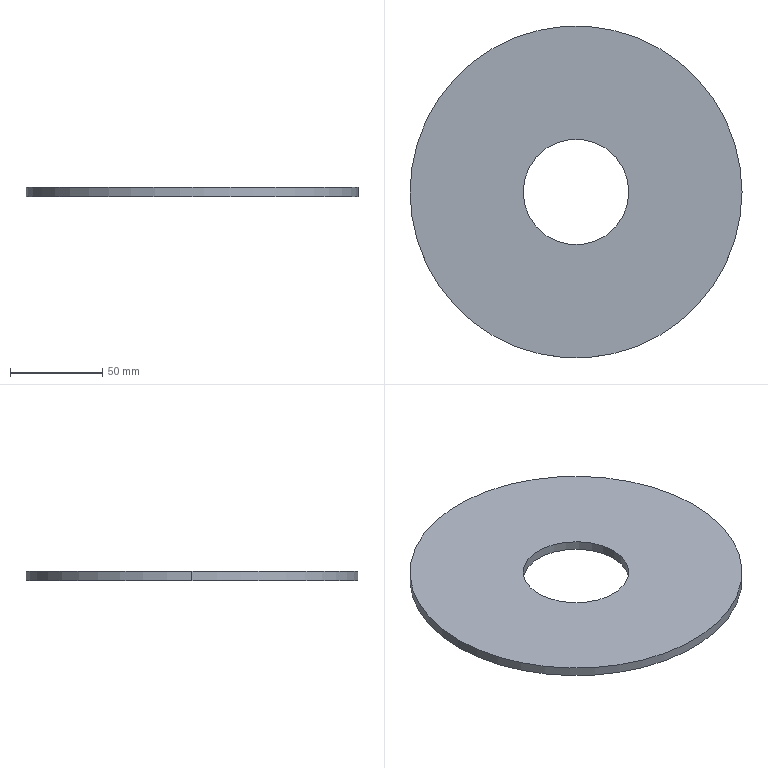Part | SolidWorks | features FlatPattern 1, SMBaseFlange 1, SheetMetal 1 | 1 solid | 6 faces | box 180 x 180 x 5 mm | volume 114341 mm3 | cylinder 4 | plane 2 | commonest cylinder face diameters 57.3 x2 180 x2
STEP:
#1=CARTESIAN_POINT('',(-38.194,24.146,5.));
#2=VERTEX_POINT('',#1);
#3=CARTESIAN_POINT('',(19.106,24.146,5.));
#4=VERTEX_POINT('',#3);
#5=CARTESIAN_POINT('',(-9.544,24.146,5.));
#6=DIRECTION('',(0.,0.,1.));
#7=DIRECTION('',(1.,0.,0.));
#8=AXIS2_PLACEMENT_3D('',#5,#6,#7);
#9=CIRCLE('',#8,28.65);
#10=EDGE_CURVE('',#2,#4,#9,.T.);
#11=ORIENTED_EDGE('',*,*,#10,.T.);
#12=CARTESIAN_POINT('',(19.106,24.146,0.));
#13=VERTEX_POINT('',#12);
#14=CARTESIAN_POINT('',(19.106,24.146,5.));
#15=DIRECTION('',(0.,0.,-1.));
#16=VECTOR('',#15,1000.);
#17=LINE('',#14,#16);
#18=EDGE_CURVE('',#4,#13,#17,.T.);
#19=ORIENTED_EDGE('',*,*,#18,.T.);
#20=CARTESIAN_POINT('',(-38.194,24.146,0.));
#21=VERTEX_POINT('',#20);
#22=CARTESIAN_POINT('',(-9.544,24.146,0.));
#23=DIRECTION('',(0.,0.,1.));
#24=DIRECTION('',(1.,0.,0.));
#25=AXIS2_PLACEMENT_3D('',#22,#23,#24);
#26=CIRCLE('',#25,28.65);
#27=EDGE_CURVE('',#21,#13,#26,.T.);
#28=ORIENTED_EDGE('',*,*,#27,.F.);
#29=CARTESIAN_POINT('',(-38.194,24.146,5.));
#30=DIRECTION('',(0.,0.,-1.));
#31=VECTOR('',#30,1000.);
#32=LINE('',#29,#31);
#33=EDGE_CURVE('',#2,#21,#32,.T.);
#34=ORIENTED_EDGE('',*,*,#33,.F.);
#35=EDGE_LOOP('',(#11,#19,#28,#34));
#36=FACE_OUTER_BOUND('',#35,.T.);
#37=CARTESIAN_POINT('',(-9.544,24.146,5.));
#38=DIRECTION('',(0.,0.,-1.));
#39=DIRECTION('',(-1.,0.,0.));
#40=AXIS2_PLACEMENT_3D('',#37,#38,#39);
#41=CYLINDRICAL_SURFACE('',#40,28.65);
#42=ADVANCED_FACE('',(#36),#41,.F.);
#43=CARTESIAN_POINT('',(80.456,24.146,5.));
#44=VERTEX_POINT('',#43);
#45=CARTESIAN_POINT('',(-99.544,24.146,5.));
#46=VERTEX_POINT('',#45);
#47=CARTESIAN_POINT('',(-9.544,24.146,5.));
#48=DIRECTION('',(0.,0.,1.));
#49=DIRECTION('',(1.,0.,0.));
#50=AXIS2_PLACEMENT_3D('',#47,#48,#49);
#51=CIRCLE('',#50,90.);
#52=EDGE_CURVE('',#44,#46,#51,.T.);
#53=ORIENTED_EDGE('',*,*,#52,.F.);
#54=CARTESIAN_POINT('',(80.456,24.146,0.));
#55=VERTEX_POINT('',#54);
#56=CARTESIAN_POINT('',(80.456,24.146,5.));
#57=DIRECTION('',(0.,0.,-1.));
#58=VECTOR('',#57,1000.);
#59=LINE('',#56,#58);
#60=EDGE_CURVE('',#44,#55,#59,.T.);
#61=ORIENTED_EDGE('',*,*,#60,.T.);
#62=CARTESIAN_POINT('',(-99.544,24.146,0.));
#63=VERTEX_POINT('',#62);
#64=CARTESIAN_POINT('',(-9.544,24.146,0.));
#65=DIRECTION('',(0.,0.,1.));
#66=DIRECTION('',(1.,0.,0.));
#67=AXIS2_PLACEMENT_3D('',#64,#65,#66);
#68=CIRCLE('',#67,90.);
#69=EDGE_CURVE('',#55,#63,#68,.T.);
#70=ORIENTED_EDGE('',*,*,#69,.T.);
#71=CARTESIAN_POINT('',(-99.544,24.146,5.));
#72=DIRECTION('',(0.,0.,-1.));
#73=VECTOR('',#72,1000.);
#74=LINE('',#71,#73);
#75=EDGE_CURVE('',#46,#63,#74,.T.);
#76=ORIENTED_EDGE('',*,*,#75,.F.);
#77=EDGE_LOOP('',(#53,#61,#70,#76));
#78=FACE_OUTER_BOUND('',#77,.T.);
#79=CARTESIAN_POINT('',(-9.544,24.146,5.));
#80=DIRECTION('',(0.,0.,-1.));
#81=DIRECTION('',(-1.,0.,0.));
#82=AXIS2_PLACEMENT_3D('',#79,#80,#81);
#83=CYLINDRICAL_SURFACE('',#82,90.);
#84=ADVANCED_FACE('',(#78),#83,.T.);
#85=CARTESIAN_POINT('',(-9.544,24.146,5.));
#86=DIRECTION('',(0.,0.,1.));
#87=DIRECTION('',(1.,0.,0.));
#88=AXIS2_PLACEMENT_3D('',#85,#86,#87);
#89=CIRCLE('',#88,90.);
#90=EDGE_CURVE('',#46,#44,#89,.T.);
#91=ORIENTED_EDGE('',*,*,#90,.T.);
#92=ORIENTED_EDGE('',*,*,#52,.T.);
#93=EDGE_LOOP('',(#91,#92));
#94=FACE_OUTER_BOUND('',#93,.T.);
#95=ORIENTED_EDGE('',*,*,#10,.F.);
#96=CARTESIAN_POINT('',(-9.544,24.146,5.));
#97=DIRECTION('',(0.,0.,1.));
#98=DIRECTION('',(1.,0.,0.));
#99=AXIS2_PLACEMENT_3D('',#96,#97,#98);
#100=CIRCLE('',#99,28.65);
#101=EDGE_CURVE('',#4,#2,#100,.T.);
#102=ORIENTED_EDGE('',*,*,#101,.F.);
#103=EDGE_LOOP('',(#95,#102));
#104=FACE_BOUND('',#103,.T.);
#105=CARTESIAN_POINT('',(-9.544,24.146,5.));
#106=DIRECTION('',(0.,0.,1.));
#107=DIRECTION('',(1.,0.,0.));
#108=AXIS2_PLACEMENT_3D('',#105,#106,#107);
#109=PLANE('',#108);
#110=ADVANCED_FACE('',(#94,#104),#109,.T.);
#111=CARTESIAN_POINT('',(-9.544,24.146,0.));
#112=DIRECTION('',(0.,0.,1.));
#113=DIRECTION('',(1.,0.,0.));
#114=AXIS2_PLACEMENT_3D('',#111,#112,#113);
#115=CIRCLE('',#114,90.);
#116=EDGE_CURVE('',#63,#55,#115,.T.);
#117=ORIENTED_EDGE('',*,*,#116,.F.);
#118=ORIENTED_EDGE('',*,*,#69,.F.);
#119=EDGE_LOOP('',(#117,#118));
#120=FACE_OUTER_BOUND('',#119,.T.);
#121=ORIENTED_EDGE('',*,*,#27,.T.);
#122=CARTESIAN_POINT('',(-9.544,24.146,0.));
#123=DIRECTION('',(0.,0.,1.));
#124=DIRECTION('',(1.,0.,0.));
#125=AXIS2_PLACEMENT_3D('',#122,#123,#124);
#126=CIRCLE('',#125,28.65);
#127=EDGE_CURVE('',#13,#21,#126,.T.);
#128=ORIENTED_EDGE('',*,*,#127,.T.);
#129=EDGE_LOOP('',(#121,#128));
#130=FACE_BOUND('',#129,.T.);
#131=CARTESIAN_POINT('',(-9.544,24.146,0.));
#132=DIRECTION('',(0.,0.,1.));
#133=DIRECTION('',(1.,0.,0.));
#134=AXIS2_PLACEMENT_3D('',#131,#132,#133);
#135=PLANE('',#134);
#136=ADVANCED_FACE('',(#120,#130),#135,.F.);
#137=ORIENTED_EDGE('',*,*,#60,.F.);
#138=ORIENTED_EDGE('',*,*,#90,.F.);
#139=ORIENTED_EDGE('',*,*,#75,.T.);
#140=ORIENTED_EDGE('',*,*,#116,.T.);
#141=EDGE_LOOP('',(#137,#138,#139,#140));
#142=FACE_OUTER_BOUND('',#141,.T.);
#143=CARTESIAN_POINT('',(-9.544,24.146,5.));
#144=DIRECTION('',(0.,0.,-1.));
#145=DIRECTION('',(-1.,0.,0.));
#146=AXIS2_PLACEMENT_3D('',#143,#144,#145);
#147=CYLINDRICAL_SURFACE('',#146,90.);
#148=ADVANCED_FACE('',(#142),#147,.T.);
#149=ORIENTED_EDGE('',*,*,#18,.F.);
#150=ORIENTED_EDGE('',*,*,#101,.T.);
#151=ORIENTED_EDGE('',*,*,#33,.T.);
#152=ORIENTED_EDGE('',*,*,#127,.F.);
#153=EDGE_LOOP('',(#149,#150,#151,#152));
#154=FACE_OUTER_BOUND('',#153,.T.);
#155=CARTESIAN_POINT('',(-9.544,24.146,5.));
#156=DIRECTION('',(0.,0.,-1.));
#157=DIRECTION('',(-1.,0.,0.));
#158=AXIS2_PLACEMENT_3D('',#155,#156,#157);
#159=CYLINDRICAL_SURFACE('',#158,28.65);
#160=ADVANCED_FACE('',(#154),#159,.F.);
#161=CLOSED_SHELL('',(#42,#84,#110,#136,#148,#160));
#162=MANIFOLD_SOLID_BREP('',#161);
#163=CARTESIAN_POINT('',(0.,0.,0.));
#164=DIRECTION('',(0.,0.,1.));
#165=DIRECTION('',(1.,0.,0.));
#166=AXIS2_PLACEMENT_3D('',#163,#164,#165);
#167=(LENGTH_UNIT()NAMED_UNIT(*)SI_UNIT(.MILLI.,.METRE.));
#168=UNCERTAINTY_MEASURE_WITH_UNIT(LENGTH_MEASURE(0.00001),#167,'','');
#169=(NAMED_UNIT(*)PLANE_ANGLE_UNIT()SI_UNIT($,.RADIAN.));
#170=(NAMED_UNIT(*)SI_UNIT($,.STERADIAN.)SOLID_ANGLE_UNIT());
#171=(GEOMETRIC_REPRESENTATION_CONTEXT(3)GLOBAL_UNCERTAINTY_ASSIGNED_CONTEXT((#168))GLOBAL_UNIT_ASSIGNED_CONTEXT((#167,#169,#170))REPRESENTATION_CONTEXT('',''));
#172=ADVANCED_BREP_SHAPE_REPRESENTATION('',(#162,#166),#171);